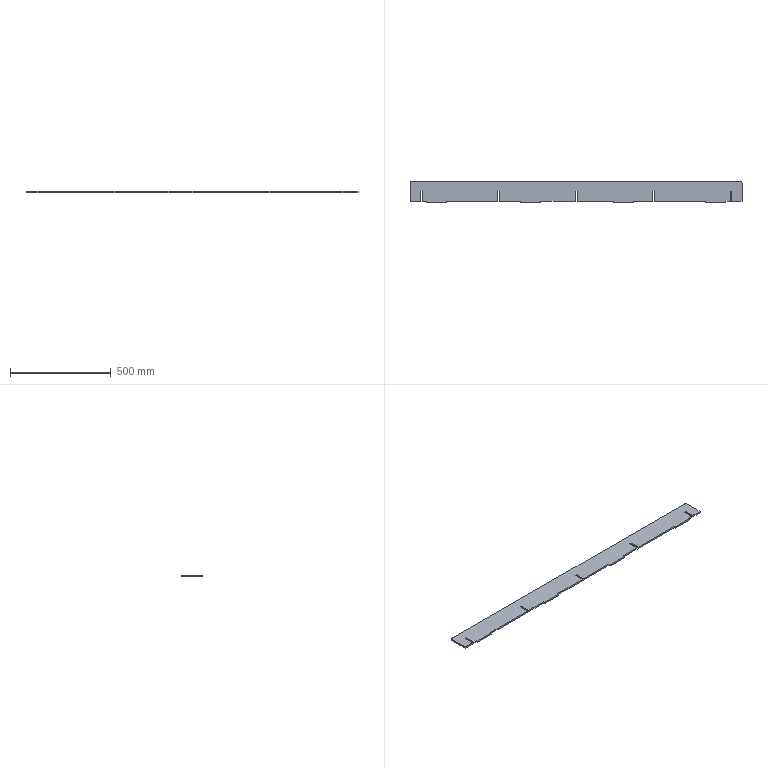Part | SolidWorks | features FlatPattern 1, SMBaseFlange 1, SheetMetal 1 | 1 solid | 44 faces | box 1650 x 107.5 x 8 mm | volume 1327497 mm3 | plane 42 | cylinder 2 | commonest cylinder face diameters 20 x2
STEP:
#1=CARTESIAN_POINT('',(838.136,-1279.45,0.));
#2=VERTEX_POINT('',#1);
#3=CARTESIAN_POINT('',(888.136,-1279.45,0.));
#4=VERTEX_POINT('',#3);
#5=CARTESIAN_POINT('',(838.136,-1279.45,0.));
#6=DIRECTION('',(1.,0.,0.));
#7=VECTOR('',#6,1000.);
#8=LINE('',#5,#7);
#9=EDGE_CURVE('',#2,#4,#8,.T.);
#10=ORIENTED_EDGE('',*,*,#9,.F.);
#11=CARTESIAN_POINT('',(838.136,-1279.45,-8.));
#12=VERTEX_POINT('',#11);
#13=CARTESIAN_POINT('',(838.136,-1279.45,-8.));
#14=DIRECTION('',(0.,0.,1.));
#15=VECTOR('',#14,1000.);
#16=LINE('',#13,#15);
#17=EDGE_CURVE('',#12,#2,#16,.T.);
#18=ORIENTED_EDGE('',*,*,#17,.F.);
#19=CARTESIAN_POINT('',(888.136,-1279.45,-8.));
#20=VERTEX_POINT('',#19);
#21=CARTESIAN_POINT('',(838.136,-1279.45,-8.));
#22=DIRECTION('',(1.,0.,0.));
#23=VECTOR('',#22,1000.);
#24=LINE('',#21,#23);
#25=EDGE_CURVE('',#12,#20,#24,.T.);
#26=ORIENTED_EDGE('',*,*,#25,.T.);
#27=CARTESIAN_POINT('',(888.136,-1279.45,-8.));
#28=DIRECTION('',(0.,0.,1.));
#29=VECTOR('',#28,1000.);
#30=LINE('',#27,#29);
#31=EDGE_CURVE('',#20,#4,#30,.T.);
#32=ORIENTED_EDGE('',*,*,#31,.T.);
#33=EDGE_LOOP('',(#10,#18,#26,#32));
#34=FACE_OUTER_BOUND('',#33,.T.);
#35=CARTESIAN_POINT('',(838.136,-1279.45,-8.));
#36=DIRECTION('',(0.,-1.,0.));
#37=DIRECTION('',(1.,0.,0.));
#38=AXIS2_PLACEMENT_3D('',#35,#36,#37);
#39=PLANE('',#38);
#40=ADVANCED_FACE('',(#34),#39,.T.);
#41=CARTESIAN_POINT('',(838.136,-1228.95,0.));
#42=VERTEX_POINT('',#41);
#43=CARTESIAN_POINT('',(838.136,-1279.45,0.));
#44=DIRECTION('',(0.,-1.,0.));
#45=VECTOR('',#44,1000.);
#46=LINE('',#43,#45);
#47=EDGE_CURVE('',#42,#2,#46,.T.);
#48=ORIENTED_EDGE('',*,*,#47,.F.);
#49=CARTESIAN_POINT('',(838.136,-1228.95,-8.));
#50=VERTEX_POINT('',#49);
#51=CARTESIAN_POINT('',(838.136,-1228.95,-8.));
#52=DIRECTION('',(0.,0.,1.));
#53=VECTOR('',#52,1000.);
#54=LINE('',#51,#53);
#55=EDGE_CURVE('',#50,#42,#54,.T.);
#56=ORIENTED_EDGE('',*,*,#55,.F.);
#57=CARTESIAN_POINT('',(838.136,-1279.45,-8.));
#58=DIRECTION('',(0.,-1.,0.));
#59=VECTOR('',#58,1000.);
#60=LINE('',#57,#59);
#61=EDGE_CURVE('',#50,#12,#60,.T.);
#62=ORIENTED_EDGE('',*,*,#61,.T.);
#63=ORIENTED_EDGE('',*,*,#17,.T.);
#64=EDGE_LOOP('',(#48,#56,#62,#63));
#65=FACE_OUTER_BOUND('',#64,.T.);
#66=CARTESIAN_POINT('',(838.136,-1279.45,-8.));
#67=DIRECTION('',(-1.,0.,0.));
#68=DIRECTION('',(0.,-1.,0.));
#69=AXIS2_PLACEMENT_3D('',#66,#67,#68);
#70=PLANE('',#69);
#71=ADVANCED_FACE('',(#65),#70,.T.);
#72=CARTESIAN_POINT('',(830.136,-1228.95,0.));
#73=VERTEX_POINT('',#72);
#74=CARTESIAN_POINT('',(838.136,-1228.95,0.));
#75=DIRECTION('',(1.,0.,0.));
#76=VECTOR('',#75,1000.);
#77=LINE('',#74,#76);
#78=EDGE_CURVE('',#73,#42,#77,.T.);
#79=ORIENTED_EDGE('',*,*,#78,.F.);
#80=CARTESIAN_POINT('',(830.136,-1228.95,-8.));
#81=VERTEX_POINT('',#80);
#82=CARTESIAN_POINT('',(830.136,-1228.95,-8.));
#83=DIRECTION('',(0.,0.,1.));
#84=VECTOR('',#83,1000.);
#85=LINE('',#82,#84);
#86=EDGE_CURVE('',#81,#73,#85,.T.);
#87=ORIENTED_EDGE('',*,*,#86,.F.);
#88=CARTESIAN_POINT('',(838.136,-1228.95,-8.));
#89=DIRECTION('',(1.,0.,0.));
#90=VECTOR('',#89,1000.);
#91=LINE('',#88,#90);
#92=EDGE_CURVE('',#81,#50,#91,.T.);
#93=ORIENTED_EDGE('',*,*,#92,.T.);
#94=ORIENTED_EDGE('',*,*,#55,.T.);
#95=EDGE_LOOP('',(#79,#87,#93,#94));
#96=FACE_OUTER_BOUND('',#95,.T.);
#97=CARTESIAN_POINT('',(838.136,-1228.95,-8.));
#98=DIRECTION('',(0.,-1.,0.));
#99=DIRECTION('',(0.,0.,-1.));
#100=AXIS2_PLACEMENT_3D('',#97,#98,#99);
#101=PLANE('',#100);
#102=ADVANCED_FACE('',(#96),#101,.T.);
#103=CARTESIAN_POINT('',(830.136,-1279.45,0.));
#104=VERTEX_POINT('',#103);
#105=CARTESIAN_POINT('',(830.136,-1228.95,0.));
#106=DIRECTION('',(0.,1.,0.));
#107=VECTOR('',#106,1000.);
#108=LINE('',#105,#107);
#109=EDGE_CURVE('',#104,#73,#108,.T.);
#110=ORIENTED_EDGE('',*,*,#109,.F.);
#111=CARTESIAN_POINT('',(830.136,-1279.45,-8.));
#112=VERTEX_POINT('',#111);
#113=CARTESIAN_POINT('',(830.136,-1279.45,-8.));
#114=DIRECTION('',(0.,0.,1.));
#115=VECTOR('',#114,1000.);
#116=LINE('',#113,#115);
#117=EDGE_CURVE('',#112,#104,#116,.T.);
#118=ORIENTED_EDGE('',*,*,#117,.F.);
#119=CARTESIAN_POINT('',(830.136,-1228.95,-8.));
#120=DIRECTION('',(0.,1.,0.));
#121=VECTOR('',#120,1000.);
#122=LINE('',#119,#121);
#123=EDGE_CURVE('',#112,#81,#122,.T.);
#124=ORIENTED_EDGE('',*,*,#123,.T.);
#125=ORIENTED_EDGE('',*,*,#86,.T.);
#126=EDGE_LOOP('',(#110,#118,#124,#125));
#127=FACE_OUTER_BOUND('',#126,.T.);
#128=CARTESIAN_POINT('',(830.136,-1228.95,-8.));
#129=DIRECTION('',(1.,0.,0.));
#130=DIRECTION('',(0.,0.,-1.));
#131=AXIS2_PLACEMENT_3D('',#128,#129,#130);
#132=PLANE('',#131);
#133=ADVANCED_FACE('',(#127),#132,.T.);
#134=CARTESIAN_POINT('',(808.136,-1279.45,0.));
#135=VERTEX_POINT('',#134);
#136=CARTESIAN_POINT('',(808.136,-1279.45,0.));
#137=DIRECTION('',(1.,0.,0.));
#138=VECTOR('',#137,1000.);
#139=LINE('',#136,#138);
#140=EDGE_CURVE('',#135,#104,#139,.T.);
#141=ORIENTED_EDGE('',*,*,#140,.F.);
#142=CARTESIAN_POINT('',(808.136,-1279.45,-8.));
#143=VERTEX_POINT('',#142);
#144=CARTESIAN_POINT('',(808.136,-1279.45,-8.));
#145=DIRECTION('',(0.,0.,1.));
#146=VECTOR('',#145,1000.);
#147=LINE('',#144,#146);
#148=EDGE_CURVE('',#143,#135,#147,.T.);
#149=ORIENTED_EDGE('',*,*,#148,.F.);
#150=CARTESIAN_POINT('',(808.136,-1279.45,-8.));
#151=DIRECTION('',(1.,0.,0.));
#152=VECTOR('',#151,1000.);
#153=LINE('',#150,#152);
#154=EDGE_CURVE('',#143,#112,#153,.T.);
#155=ORIENTED_EDGE('',*,*,#154,.T.);
#156=ORIENTED_EDGE('',*,*,#117,.T.);
#157=EDGE_LOOP('',(#141,#149,#155,#156));
#158=FACE_OUTER_BOUND('',#157,.T.);
#159=CARTESIAN_POINT('',(808.136,-1279.45,-8.));
#160=DIRECTION('',(0.,-1.,0.));
#161=DIRECTION('',(1.,0.,0.));
#162=AXIS2_PLACEMENT_3D('',#159,#160,#161);
#163=PLANE('',#162);
#164=ADVANCED_FACE('',(#158),#163,.T.);
#165=CARTESIAN_POINT('',(808.136,-1286.95,0.));
#166=VERTEX_POINT('',#165);
#167=CARTESIAN_POINT('',(808.136,-1279.45,0.));
#168=DIRECTION('',(0.,1.,0.));
#169=VECTOR('',#168,1000.);
#170=LINE('',#167,#169);
#171=EDGE_CURVE('',#166,#135,#170,.T.);
#172=ORIENTED_EDGE('',*,*,#171,.F.);
#173=CARTESIAN_POINT('',(808.136,-1286.95,-8.));
#174=VERTEX_POINT('',#173);
#175=CARTESIAN_POINT('',(808.136,-1286.95,-8.));
#176=DIRECTION('',(0.,0.,1.));
#177=VECTOR('',#176,1000.);
#178=LINE('',#175,#177);
#179=EDGE_CURVE('',#174,#166,#178,.T.);
#180=ORIENTED_EDGE('',*,*,#179,.F.);
#181=CARTESIAN_POINT('',(808.136,-1279.45,-8.));
#182=DIRECTION('',(0.,1.,0.));
#183=VECTOR('',#182,1000.);
#184=LINE('',#181,#183);
#185=EDGE_CURVE('',#174,#143,#184,.T.);
#186=ORIENTED_EDGE('',*,*,#185,.T.);
#187=ORIENTED_EDGE('',*,*,#148,.T.);
#188=EDGE_LOOP('',(#172,#180,#186,#187));
#189=FACE_OUTER_BOUND('',#188,.T.);
#190=CARTESIAN_POINT('',(808.136,-1279.45,-8.));
#191=DIRECTION('',(1.,0.,0.));
#192=DIRECTION('',(0.,0.,-1.));
#193=AXIS2_PLACEMENT_3D('',#190,#191,#192);
#194=PLANE('',#193);
#195=ADVANCED_FACE('',(#189),#194,.T.);
#196=CARTESIAN_POINT('',(708.136,-1286.95,0.));
#197=VERTEX_POINT('',#196);
#198=CARTESIAN_POINT('',(808.136,-1286.95,0.));
#199=DIRECTION('',(1.,0.,0.));
#200=VECTOR('',#199,1000.);
#201=LINE('',#198,#200);
#202=EDGE_CURVE('',#197,#166,#201,.T.);
#203=ORIENTED_EDGE('',*,*,#202,.F.);
#204=CARTESIAN_POINT('',(708.136,-1286.95,-8.));
#205=VERTEX_POINT('',#204);
#206=CARTESIAN_POINT('',(708.136,-1286.95,-8.));
#207=DIRECTION('',(0.,0.,1.));
#208=VECTOR('',#207,1000.);
#209=LINE('',#206,#208);
#210=EDGE_CURVE('',#205,#197,#209,.T.);
#211=ORIENTED_EDGE('',*,*,#210,.F.);
#212=CARTESIAN_POINT('',(808.136,-1286.95,-8.));
#213=DIRECTION('',(1.,0.,0.));
#214=VECTOR('',#213,1000.);
#215=LINE('',#212,#214);
#216=EDGE_CURVE('',#205,#174,#215,.T.);
#217=ORIENTED_EDGE('',*,*,#216,.T.);
#218=ORIENTED_EDGE('',*,*,#179,.T.);
#219=EDGE_LOOP('',(#203,#211,#217,#218));
#220=FACE_OUTER_BOUND('',#219,.T.);
#221=CARTESIAN_POINT('',(808.136,-1286.95,-8.));
#222=DIRECTION('',(0.,-1.,0.));
#223=DIRECTION('',(1.,0.,0.));
#224=AXIS2_PLACEMENT_3D('',#221,#222,#223);
#225=PLANE('',#224);
#226=ADVANCED_FACE('',(#220),#225,.T.);
#227=CARTESIAN_POINT('',(708.136,-1279.45,0.));
#228=VERTEX_POINT('',#227);
#229=CARTESIAN_POINT('',(708.136,-1286.95,0.));
#230=DIRECTION('',(0.,-1.,0.));
#231=VECTOR('',#230,1000.);
#232=LINE('',#229,#231);
#233=EDGE_CURVE('',#228,#197,#232,.T.);
#234=ORIENTED_EDGE('',*,*,#233,.F.);
#235=CARTESIAN_POINT('',(708.136,-1279.45,-8.));
#236=VERTEX_POINT('',#235);
#237=CARTESIAN_POINT('',(708.136,-1279.45,-8.));
#238=DIRECTION('',(0.,0.,1.));
#239=VECTOR('',#238,1000.);
#240=LINE('',#237,#239);
#241=EDGE_CURVE('',#236,#228,#240,.T.);
#242=ORIENTED_EDGE('',*,*,#241,.F.);
#243=CARTESIAN_POINT('',(708.136,-1286.95,-8.));
#244=DIRECTION('',(0.,-1.,0.));
#245=VECTOR('',#244,1000.);
#246=LINE('',#243,#245);
#247=EDGE_CURVE('',#236,#205,#246,.T.);
#248=ORIENTED_EDGE('',*,*,#247,.T.);
#249=ORIENTED_EDGE('',*,*,#210,.T.);
#250=EDGE_LOOP('',(#234,#242,#248,#249));
#251=FACE_OUTER_BOUND('',#250,.T.);
#252=CARTESIAN_POINT('',(708.136,-1286.95,-8.));
#253=DIRECTION('',(-1.,0.,0.));
#254=DIRECTION('',(0.,0.,1.));
#255=AXIS2_PLACEMENT_3D('',#252,#253,#254);
#256=PLANE('',#255);
#257=ADVANCED_FACE('',(#251),#256,.T.);
#258=CARTESIAN_POINT('',(453.136,-1279.45,0.));
#259=VERTEX_POINT('',#258);
#260=CARTESIAN_POINT('',(453.136,-1279.45,0.));
#261=DIRECTION('',(1.,0.,0.));
#262=VECTOR('',#261,1000.);
#263=LINE('',#260,#262);
#264=EDGE_CURVE('',#259,#228,#263,.T.);
#265=ORIENTED_EDGE('',*,*,#264,.F.);
#266=CARTESIAN_POINT('',(453.136,-1279.45,-8.));
#267=VERTEX_POINT('',#266);
#268=CARTESIAN_POINT('',(453.136,-1279.45,-8.));
#269=DIRECTION('',(0.,0.,1.));
#270=VECTOR('',#269,1000.);
#271=LINE('',#268,#270);
#272=EDGE_CURVE('',#267,#259,#271,.T.);
#273=ORIENTED_EDGE('',*,*,#272,.F.);
#274=CARTESIAN_POINT('',(453.136,-1279.45,-8.));
#275=DIRECTION('',(1.,0.,0.));
#276=VECTOR('',#275,1000.);
#277=LINE('',#274,#276);
#278=EDGE_CURVE('',#267,#236,#277,.T.);
#279=ORIENTED_EDGE('',*,*,#278,.T.);
#280=ORIENTED_EDGE('',*,*,#241,.T.);
#281=EDGE_LOOP('',(#265,#273,#279,#280));
#282=FACE_OUTER_BOUND('',#281,.T.);
#283=CARTESIAN_POINT('',(453.136,-1279.45,-8.));
#284=DIRECTION('',(0.,-1.,0.));
#285=DIRECTION('',(1.,0.,0.));
#286=AXIS2_PLACEMENT_3D('',#283,#284,#285);
#287=PLANE('',#286);
#288=ADVANCED_FACE('',(#282),#287,.T.);
#289=CARTESIAN_POINT('',(453.136,-1228.95,0.));
#290=VERTEX_POINT('',#289);
#291=CARTESIAN_POINT('',(453.136,-1279.45,0.));
#292=DIRECTION('',(0.,-1.,0.));
#293=VECTOR('',#292,1000.);
#294=LINE('',#291,#293);
#295=EDGE_CURVE('',#290,#259,#294,.T.);
#296=ORIENTED_EDGE('',*,*,#295,.F.);
#297=CARTESIAN_POINT('',(453.136,-1228.95,-8.));
#298=VERTEX_POINT('',#297);
#299=CARTESIAN_POINT('',(453.136,-1228.95,-8.));
#300=DIRECTION('',(0.,0.,1.));
#301=VECTOR('',#300,1000.);
#302=LINE('',#299,#301);
#303=EDGE_CURVE('',#298,#290,#302,.T.);
#304=ORIENTED_EDGE('',*,*,#303,.F.);
#305=CARTESIAN_POINT('',(453.136,-1279.45,-8.));
#306=DIRECTION('',(0.,-1.,0.));
#307=VECTOR('',#306,1000.);
#308=LINE('',#305,#307);
#309=EDGE_CURVE('',#298,#267,#308,.T.);
#310=ORIENTED_EDGE('',*,*,#309,.T.);
#311=ORIENTED_EDGE('',*,*,#272,.T.);
#312=EDGE_LOOP('',(#296,#304,#310,#311));
#313=FACE_OUTER_BOUND('',#312,.T.);
#314=CARTESIAN_POINT('',(453.136,-1279.45,-8.));
#315=DIRECTION('',(-1.,0.,0.));
#316=DIRECTION('',(0.,0.,1.));
#317=AXIS2_PLACEMENT_3D('',#314,#315,#316);
#318=PLANE('',#317);
#319=ADVANCED_FACE('',(#313),#318,.T.);
#320=CARTESIAN_POINT('',(445.136,-1228.95,0.));
#321=VERTEX_POINT('',#320);
#322=CARTESIAN_POINT('',(453.136,-1228.95,0.));
#323=DIRECTION('',(1.,0.,0.));
#324=VECTOR('',#323,1000.);
#325=LINE('',#322,#324);
#326=EDGE_CURVE('',#321,#290,#325,.T.);
#327=ORIENTED_EDGE('',*,*,#326,.F.);
#328=CARTESIAN_POINT('',(445.136,-1228.95,-8.));
#329=VERTEX_POINT('',#328);
#330=CARTESIAN_POINT('',(445.136,-1228.95,-8.));
#331=DIRECTION('',(0.,0.,1.));
#332=VECTOR('',#331,1000.);
#333=LINE('',#330,#332);
#334=EDGE_CURVE('',#329,#321,#333,.T.);
#335=ORIENTED_EDGE('',*,*,#334,.F.);
#336=CARTESIAN_POINT('',(453.136,-1228.95,-8.));
#337=DIRECTION('',(1.,0.,0.));
#338=VECTOR('',#337,1000.);
#339=LINE('',#336,#338);
#340=EDGE_CURVE('',#329,#298,#339,.T.);
#341=ORIENTED_EDGE('',*,*,#340,.T.);
#342=ORIENTED_EDGE('',*,*,#303,.T.);
#343=EDGE_LOOP('',(#327,#335,#341,#342));
#344=FACE_OUTER_BOUND('',#343,.T.);
#345=CARTESIAN_POINT('',(453.136,-1228.95,-8.));
#346=DIRECTION('',(0.,-1.,0.));
#347=DIRECTION('',(0.,0.,-1.));
#348=AXIS2_PLACEMENT_3D('',#345,#346,#347);
#349=PLANE('',#348);
#350=ADVANCED_FACE('',(#344),#349,.T.);
#351=CARTESIAN_POINT('',(445.136,-1279.45,0.));
#352=VERTEX_POINT('',#351);
#353=CARTESIAN_POINT('',(445.136,-1228.95,0.));
#354=DIRECTION('',(0.,1.,0.));
#355=VECTOR('',#354,1000.);
#356=LINE('',#353,#355);
#357=EDGE_CURVE('',#352,#321,#356,.T.);
#358=ORIENTED_EDGE('',*,*,#357,.F.);
#359=CARTESIAN_POINT('',(445.136,-1279.45,-8.));
#360=VERTEX_POINT('',#359);
#361=CARTESIAN_POINT('',(445.136,-1279.45,-8.));
#362=DIRECTION('',(0.,0.,1.));
#363=VECTOR('',#362,1000.);
#364=LINE('',#361,#363);
#365=EDGE_CURVE('',#360,#352,#364,.T.);
#366=ORIENTED_EDGE('',*,*,#365,.F.);
#367=CARTESIAN_POINT('',(445.136,-1228.95,-8.));
#368=DIRECTION('',(0.,1.,0.));
#369=VECTOR('',#368,1000.);
#370=LINE('',#367,#369);
#371=EDGE_CURVE('',#360,#329,#370,.T.);
#372=ORIENTED_EDGE('',*,*,#371,.T.);
#373=ORIENTED_EDGE('',*,*,#334,.T.);
#374=EDGE_LOOP('',(#358,#366,#372,#373));
#375=FACE_OUTER_BOUND('',#374,.T.);
#376=CARTESIAN_POINT('',(445.136,-1228.95,-8.));
#377=DIRECTION('',(1.,0.,0.));
#378=DIRECTION('',(0.,0.,-1.));
#379=AXIS2_PLACEMENT_3D('',#376,#377,#378);
#380=PLANE('',#379);
#381=ADVANCED_FACE('',(#375),#380,.T.);
#382=CARTESIAN_POINT('',(348.136,-1279.45,0.));
#383=VERTEX_POINT('',#382);
#384=CARTESIAN_POINT('',(348.136,-1279.45,0.));
#385=DIRECTION('',(1.,0.,0.));
#386=VECTOR('',#385,1000.);
#387=LINE('',#384,#386);
#388=EDGE_CURVE('',#383,#352,#387,.T.);
#389=ORIENTED_EDGE('',*,*,#388,.F.);
#390=CARTESIAN_POINT('',(348.136,-1279.45,-8.));
#391=VERTEX_POINT('',#390);
#392=CARTESIAN_POINT('',(348.136,-1279.45,-8.));
#393=DIRECTION('',(0.,0.,1.));
#394=VECTOR('',#393,1000.);
#395=LINE('',#392,#394);
#396=EDGE_CURVE('',#391,#383,#395,.T.);
#397=ORIENTED_EDGE('',*,*,#396,.F.);
#398=CARTESIAN_POINT('',(348.136,-1279.45,-8.));
#399=DIRECTION('',(1.,0.,0.));
#400=VECTOR('',#399,1000.);
#401=LINE('',#398,#400);
#402=EDGE_CURVE('',#391,#360,#401,.T.);
#403=ORIENTED_EDGE('',*,*,#402,.T.);
#404=ORIENTED_EDGE('',*,*,#365,.T.);
#405=EDGE_LOOP('',(#389,#397,#403,#404));
#406=FACE_OUTER_BOUND('',#405,.T.);
#407=CARTESIAN_POINT('',(348.136,-1279.45,-8.));
#408=DIRECTION('',(0.,-1.,0.));
#409=DIRECTION('',(1.,0.,0.));
#410=AXIS2_PLACEMENT_3D('',#407,#408,#409);
#411=PLANE('',#410);
#412=ADVANCED_FACE('',(#406),#411,.T.);
#413=CARTESIAN_POINT('',(348.136,-1286.95,0.));
#414=VERTEX_POINT('',#413);
#415=CARTESIAN_POINT('',(348.136,-1279.45,0.));
#416=DIRECTION('',(0.,1.,0.));
#417=VECTOR('',#416,1000.);
#418=LINE('',#415,#417);
#419=EDGE_CURVE('',#414,#383,#418,.T.);
#420=ORIENTED_EDGE('',*,*,#419,.F.);
#421=CARTESIAN_POINT('',(348.136,-1286.95,-8.));
#422=VERTEX_POINT('',#421);
#423=CARTESIAN_POINT('',(348.136,-1286.95,-8.));
#424=DIRECTION('',(0.,0.,1.));
#425=VECTOR('',#424,1000.);
#426=LINE('',#423,#425);
#427=EDGE_CURVE('',#422,#414,#426,.T.);
#428=ORIENTED_EDGE('',*,*,#427,.F.);
#429=CARTESIAN_POINT('',(348.136,-1279.45,-8.));
#430=DIRECTION('',(0.,1.,0.));
#431=VECTOR('',#430,1000.);
#432=LINE('',#429,#431);
#433=EDGE_CURVE('',#422,#391,#432,.T.);
#434=ORIENTED_EDGE('',*,*,#433,.T.);
#435=ORIENTED_EDGE('',*,*,#396,.T.);
#436=EDGE_LOOP('',(#420,#428,#434,#435));
#437=FACE_OUTER_BOUND('',#436,.T.);
#438=CARTESIAN_POINT('',(348.136,-1279.45,-8.));
#439=DIRECTION('',(1.,0.,0.));
#440=DIRECTION('',(0.,0.,-1.));
#441=AXIS2_PLACEMENT_3D('',#438,#439,#440);
#442=PLANE('',#441);
#443=ADVANCED_FACE('',(#437),#442,.T.);
#444=CARTESIAN_POINT('',(248.136,-1286.95,0.));
#445=VERTEX_POINT('',#444);
#446=CARTESIAN_POINT('',(348.136,-1286.95,0.));
#447=DIRECTION('',(1.,0.,0.));
#448=VECTOR('',#447,1000.);
#449=LINE('',#446,#448);
#450=EDGE_CURVE('',#445,#414,#449,.T.);
#451=ORIENTED_EDGE('',*,*,#450,.F.);
#452=CARTESIAN_POINT('',(248.136,-1286.95,-8.));
#453=VERTEX_POINT('',#452);
#454=CARTESIAN_POINT('',(248.136,-1286.95,-8.));
#455=DIRECTION('',(0.,0.,1.));
#456=VECTOR('',#455,1000.);
#457=LINE('',#454,#456);
#458=EDGE_CURVE('',#453,#445,#457,.T.);
#459=ORIENTED_EDGE('',*,*,#458,.F.);
#460=CARTESIAN_POINT('',(348.136,-1286.95,-8.));
#461=DIRECTION('',(1.,0.,0.));
#462=VECTOR('',#461,1000.);
#463=LINE('',#460,#462);
#464=EDGE_CURVE('',#453,#422,#463,.T.);
#465=ORIENTED_EDGE('',*,*,#464,.T.);
#466=ORIENTED_EDGE('',*,*,#427,.T.);
#467=EDGE_LOOP('',(#451,#459,#465,#466));
#468=FACE_OUTER_BOUND('',#467,.T.);
#469=CARTESIAN_POINT('',(348.136,-1286.95,-8.));
#470=DIRECTION('',(0.,-1.,0.));
#471=DIRECTION('',(0.,0.,-1.));
#472=AXIS2_PLACEMENT_3D('',#469,#470,#471);
#473=PLANE('',#472);
#474=ADVANCED_FACE('',(#468),#473,.T.);
#475=CARTESIAN_POINT('',(248.136,-1279.45,0.));
#476=VERTEX_POINT('',#475);
#477=CARTESIAN_POINT('',(248.136,-1286.95,0.));
#478=DIRECTION('',(0.,-1.,0.));
#479=VECTOR('',#478,1000.);
#480=LINE('',#477,#479);
#481=EDGE_CURVE('',#476,#445,#480,.T.);
#482=ORIENTED_EDGE('',*,*,#481,.F.);
#483=CARTESIAN_POINT('',(248.136,-1279.45,-8.));
#484=VERTEX_POINT('',#483);
#485=CARTESIAN_POINT('',(248.136,-1279.45,-8.));
#486=DIRECTION('',(0.,0.,1.));
#487=VECTOR('',#486,1000.);
#488=LINE('',#485,#487);
#489=EDGE_CURVE('',#484,#476,#488,.T.);
#490=ORIENTED_EDGE('',*,*,#489,.F.);
#491=CARTESIAN_POINT('',(248.136,-1286.95,-8.));
#492=DIRECTION('',(0.,-1.,0.));
#493=VECTOR('',#492,1000.);
#494=LINE('',#491,#493);
#495=EDGE_CURVE('',#484,#453,#494,.T.);
#496=ORIENTED_EDGE('',*,*,#495,.T.);
#497=ORIENTED_EDGE('',*,*,#458,.T.);
#498=EDGE_LOOP('',(#482,#490,#496,#497));
#499=FACE_OUTER_BOUND('',#498,.T.);
#500=CARTESIAN_POINT('',(248.136,-1286.95,-8.));
#501=DIRECTION('',(-1.,0.,0.));
#502=DIRECTION('',(0.,0.,1.));
#503=AXIS2_PLACEMENT_3D('',#500,#501,#502);
#504=PLANE('',#503);
#505=ADVANCED_FACE('',(#499),#504,.T.);
#506=CARTESIAN_POINT('',(68.136,-1279.45,0.));
#507=VERTEX_POINT('',#506);
#508=CARTESIAN_POINT('',(68.136,-1279.45,0.));
#509=DIRECTION('',(1.,0.,0.));
#510=VECTOR('',#509,1000.);
#511=LINE('',#508,#510);
#512=EDGE_CURVE('',#507,#476,#511,.T.);
#513=ORIENTED_EDGE('',*,*,#512,.F.);
#514=CARTESIAN_POINT('',(68.136,-1279.45,-8.));
#515=VERTEX_POINT('',#514);
#516=CARTESIAN_POINT('',(68.136,-1279.45,-8.));
#517=DIRECTION('',(0.,0.,1.));
#518=VECTOR('',#517,1000.);
#519=LINE('',#516,#518);
#520=EDGE_CURVE('',#515,#507,#519,.T.);
#521=ORIENTED_EDGE('',*,*,#520,.F.);
#522=CARTESIAN_POINT('',(68.136,-1279.45,-8.));
#523=DIRECTION('',(1.,0.,0.));
#524=VECTOR('',#523,1000.);
#525=LINE('',#522,#524);
#526=EDGE_CURVE('',#515,#484,#525,.T.);
#527=ORIENTED_EDGE('',*,*,#526,.T.);
#528=ORIENTED_EDGE('',*,*,#489,.T.);
#529=EDGE_LOOP('',(#513,#521,#527,#528));
#530=FACE_OUTER_BOUND('',#529,.T.);
#531=CARTESIAN_POINT('',(68.136,-1279.45,-8.));
#532=DIRECTION('',(0.,-1.,0.));
#533=DIRECTION('',(1.,0.,0.));
#534=AXIS2_PLACEMENT_3D('',#531,#532,#533);
#535=PLANE('',#534);
#536=ADVANCED_FACE('',(#530),#535,.T.);
#537=CARTESIAN_POINT('',(68.136,-1228.95,0.));
#538=VERTEX_POINT('',#537);
#539=CARTESIAN_POINT('',(68.136,-1279.45,0.));
#540=DIRECTION('',(0.,-1.,0.));
#541=VECTOR('',#540,1000.);
#542=LINE('',#539,#541);
#543=EDGE_CURVE('',#538,#507,#542,.T.);
#544=ORIENTED_EDGE('',*,*,#543,.F.);
#545=CARTESIAN_POINT('',(68.136,-1228.95,-8.));
#546=VERTEX_POINT('',#545);
#547=CARTESIAN_POINT('',(68.136,-1228.95,-8.));
#548=DIRECTION('',(0.,0.,1.));
#549=VECTOR('',#548,1000.);
#550=LINE('',#547,#549);
#551=EDGE_CURVE('',#546,#538,#550,.T.);
#552=ORIENTED_EDGE('',*,*,#551,.F.);
#553=CARTESIAN_POINT('',(68.136,-1279.45,-8.));
#554=DIRECTION('',(0.,-1.,0.));
#555=VECTOR('',#554,1000.);
#556=LINE('',#553,#555);
#557=EDGE_CURVE('',#546,#515,#556,.T.);
#558=ORIENTED_EDGE('',*,*,#557,.T.);
#559=ORIENTED_EDGE('',*,*,#520,.T.);
#560=EDGE_LOOP('',(#544,#552,#558,#559));
#561=FACE_OUTER_BOUND('',#560,.T.);
#562=CARTESIAN_POINT('',(68.136,-1279.45,-8.));
#563=DIRECTION('',(-1.,0.,0.));
#564=DIRECTION('',(0.,0.,1.));
#565=AXIS2_PLACEMENT_3D('',#562,#563,#564);
#566=PLANE('',#565);
#567=ADVANCED_FACE('',(#561),#566,.T.);
#568=CARTESIAN_POINT('',(60.136,-1228.95,0.));
#569=VERTEX_POINT('',#568);
#570=CARTESIAN_POINT('',(68.136,-1228.95,0.));
#571=DIRECTION('',(1.,0.,0.));
#572=VECTOR('',#571,1000.);
#573=LINE('',#570,#572);
#574=EDGE_CURVE('',#569,#538,#573,.T.);
#575=ORIENTED_EDGE('',*,*,#574,.F.);
#576=CARTESIAN_POINT('',(60.136,-1228.95,-8.));
#577=VERTEX_POINT('',#576);
#578=CARTESIAN_POINT('',(60.136,-1228.95,-8.));
#579=DIRECTION('',(0.,0.,1.));
#580=VECTOR('',#579,1000.);
#581=LINE('',#578,#580);
#582=EDGE_CURVE('',#577,#569,#581,.T.);
#583=ORIENTED_EDGE('',*,*,#582,.F.);
#584=CARTESIAN_POINT('',(68.136,-1228.95,-8.));
#585=DIRECTION('',(1.,0.,0.));
#586=VECTOR('',#585,1000.);
#587=LINE('',#584,#586);
#588=EDGE_CURVE('',#577,#546,#587,.T.);
#589=ORIENTED_EDGE('',*,*,#588,.T.);
#590=ORIENTED_EDGE('',*,*,#551,.T.);
#591=EDGE_LOOP('',(#575,#583,#589,#590));
#592=FACE_OUTER_BOUND('',#591,.T.);
#593=CARTESIAN_POINT('',(68.136,-1228.95,-8.));
#594=DIRECTION('',(0.,-1.,0.));
#595=DIRECTION('',(0.,0.,-1.));
#596=AXIS2_PLACEMENT_3D('',#593,#594,#595);
#597=PLANE('',#596);
#598=ADVANCED_FACE('',(#592),#597,.T.);
#599=CARTESIAN_POINT('',(60.136,-1279.45,0.));
#600=VERTEX_POINT('',#599);
#601=CARTESIAN_POINT('',(60.136,-1228.95,0.));
#602=DIRECTION('',(0.,1.,0.));
#603=VECTOR('',#602,1000.);
#604=LINE('',#601,#603);
#605=EDGE_CURVE('',#600,#569,#604,.T.);
#606=ORIENTED_EDGE('',*,*,#605,.F.);
#607=CARTESIAN_POINT('',(60.136,-1279.45,-8.));
#608=VERTEX_POINT('',#607);
#609=CARTESIAN_POINT('',(60.136,-1279.45,-8.));
#610=DIRECTION('',(0.,0.,1.));
#611=VECTOR('',#610,1000.);
#612=LINE('',#609,#611);
#613=EDGE_CURVE('',#608,#600,#612,.T.);
#614=ORIENTED_EDGE('',*,*,#613,.F.);
#615=CARTESIAN_POINT('',(60.136,-1228.95,-8.));
#616=DIRECTION('',(0.,1.,0.));
#617=VECTOR('',#616,1000.);
#618=LINE('',#615,#617);
#619=EDGE_CURVE('',#608,#577,#618,.T.);
#620=ORIENTED_EDGE('',*,*,#619,.T.);
#621=ORIENTED_EDGE('',*,*,#582,.T.);
#622=EDGE_LOOP('',(#606,#614,#620,#621));
#623=FACE_OUTER_BOUND('',#622,.T.);
#624=CARTESIAN_POINT('',(60.136,-1228.95,-8.));
#625=DIRECTION('',(1.,0.,0.));
#626=DIRECTION('',(0.,0.,-1.));
#627=AXIS2_PLACEMENT_3D('',#624,#625,#626);
#628=PLANE('',#627);
#629=ADVANCED_FACE('',(#623),#628,.T.);
#630=CARTESIAN_POINT('',(-111.864,-1279.45,0.));
#631=VERTEX_POINT('',#630);
#632=CARTESIAN_POINT('',(-111.864,-1279.45,0.));
#633=DIRECTION('',(1.,0.,0.));
#634=VECTOR('',#633,1000.);
#635=LINE('',#632,#634);
#636=EDGE_CURVE('',#631,#600,#635,.T.);
#637=ORIENTED_EDGE('',*,*,#636,.F.);
#638=CARTESIAN_POINT('',(-111.864,-1279.45,-8.));
#639=VERTEX_POINT('',#638);
#640=CARTESIAN_POINT('',(-111.864,-1279.45,-8.));
#641=DIRECTION('',(0.,0.,1.));
#642=VECTOR('',#641,1000.);
#643=LINE('',#640,#642);
#644=EDGE_CURVE('',#639,#631,#643,.T.);
#645=ORIENTED_EDGE('',*,*,#644,.F.);
#646=CARTESIAN_POINT('',(-111.864,-1279.45,-8.));
#647=DIRECTION('',(1.,0.,0.));
#648=VECTOR('',#647,1000.);
#649=LINE('',#646,#648);
#650=EDGE_CURVE('',#639,#608,#649,.T.);
#651=ORIENTED_EDGE('',*,*,#650,.T.);
#652=ORIENTED_EDGE('',*,*,#613,.T.);
#653=EDGE_LOOP('',(#637,#645,#651,#652));
#654=FACE_OUTER_BOUND('',#653,.T.);
#655=CARTESIAN_POINT('',(-111.864,-1279.45,-8.));
#656=DIRECTION('',(0.,-1.,0.));
#657=DIRECTION('',(1.,0.,0.));
#658=AXIS2_PLACEMENT_3D('',#655,#656,#657);
#659=PLANE('',#658);
#660=ADVANCED_FACE('',(#654),#659,.T.);
#661=CARTESIAN_POINT('',(-111.864,-1286.95,0.));
#662=VERTEX_POINT('',#661);
#663=CARTESIAN_POINT('',(-111.864,-1279.45,0.));
#664=DIRECTION('',(0.,1.,0.));
#665=VECTOR('',#664,1000.);
#666=LINE('',#663,#665);
#667=EDGE_CURVE('',#662,#631,#666,.T.);
#668=ORIENTED_EDGE('',*,*,#667,.F.);
#669=CARTESIAN_POINT('',(-111.864,-1286.95,-8.));
#670=VERTEX_POINT('',#669);
#671=CARTESIAN_POINT('',(-111.864,-1286.95,-8.));
#672=DIRECTION('',(0.,0.,1.));
#673=VECTOR('',#672,1000.);
#674=LINE('',#671,#673);
#675=EDGE_CURVE('',#670,#662,#674,.T.);
#676=ORIENTED_EDGE('',*,*,#675,.F.);
#677=CARTESIAN_POINT('',(-111.864,-1279.45,-8.));
#678=DIRECTION('',(0.,1.,0.));
#679=VECTOR('',#678,1000.);
#680=LINE('',#677,#679);
#681=EDGE_CURVE('',#670,#639,#680,.T.);
#682=ORIENTED_EDGE('',*,*,#681,.T.);
#683=ORIENTED_EDGE('',*,*,#644,.T.);
#684=EDGE_LOOP('',(#668,#676,#682,#683));
#685=FACE_OUTER_BOUND('',#684,.T.);
#686=CARTESIAN_POINT('',(-111.864,-1279.45,-8.));
#687=DIRECTION('',(1.,0.,0.));
#688=DIRECTION('',(0.,0.,-1.));
#689=AXIS2_PLACEMENT_3D('',#686,#687,#688);
#690=PLANE('',#689);
#691=ADVANCED_FACE('',(#685),#690,.T.);
#692=CARTESIAN_POINT('',(-211.864,-1286.95,0.));
#693=VERTEX_POINT('',#692);
#694=CARTESIAN_POINT('',(-111.864,-1286.95,0.));
#695=DIRECTION('',(1.,0.,0.));
#696=VECTOR('',#695,1000.);
#697=LINE('',#694,#696);
#698=EDGE_CURVE('',#693,#662,#697,.T.);
#699=ORIENTED_EDGE('',*,*,#698,.F.);
#700=CARTESIAN_POINT('',(-211.864,-1286.95,-8.));
#701=VERTEX_POINT('',#700);
#702=CARTESIAN_POINT('',(-211.864,-1286.95,-8.));
#703=DIRECTION('',(0.,0.,1.));
#704=VECTOR('',#703,1000.);
#705=LINE('',#702,#704);
#706=EDGE_CURVE('',#701,#693,#705,.T.);
#707=ORIENTED_EDGE('',*,*,#706,.F.);
#708=CARTESIAN_POINT('',(-111.864,-1286.95,-8.));
#709=DIRECTION('',(1.,0.,0.));
#710=VECTOR('',#709,1000.);
#711=LINE('',#708,#710);
#712=EDGE_CURVE('',#701,#670,#711,.T.);
#713=ORIENTED_EDGE('',*,*,#712,.T.);
#714=ORIENTED_EDGE('',*,*,#675,.T.);
#715=EDGE_LOOP('',(#699,#707,#713,#714));
#716=FACE_OUTER_BOUND('',#715,.T.);
#717=CARTESIAN_POINT('',(-111.864,-1286.95,-8.));
#718=DIRECTION('',(0.,-1.,0.));
#719=DIRECTION('',(0.,0.,-1.));
#720=AXIS2_PLACEMENT_3D('',#717,#718,#719);
#721=PLANE('',#720);
#722=ADVANCED_FACE('',(#716),#721,.T.);
#723=CARTESIAN_POINT('',(-211.864,-1279.45,0.));
#724=VERTEX_POINT('',#723);
#725=CARTESIAN_POINT('',(-211.864,-1286.95,0.));
#726=DIRECTION('',(0.,-1.,0.));
#727=VECTOR('',#726,1000.);
#728=LINE('',#725,#727);
#729=EDGE_CURVE('',#724,#693,#728,.T.);
#730=ORIENTED_EDGE('',*,*,#729,.F.);
#731=CARTESIAN_POINT('',(-211.864,-1279.45,-8.));
#732=VERTEX_POINT('',#731);
#733=CARTESIAN_POINT('',(-211.864,-1279.45,-8.));
#734=DIRECTION('',(0.,0.,1.));
#735=VECTOR('',#734,1000.);
#736=LINE('',#733,#735);
#737=EDGE_CURVE('',#732,#724,#736,.T.);
#738=ORIENTED_EDGE('',*,*,#737,.F.);
#739=CARTESIAN_POINT('',(-211.864,-1286.95,-8.));
#740=DIRECTION('',(0.,-1.,0.));
#741=VECTOR('',#740,1000.);
#742=LINE('',#739,#741);
#743=EDGE_CURVE('',#732,#701,#742,.T.);
#744=ORIENTED_EDGE('',*,*,#743,.T.);
#745=ORIENTED_EDGE('',*,*,#706,.T.);
#746=EDGE_LOOP('',(#730,#738,#744,#745));
#747=FACE_OUTER_BOUND('',#746,.T.);
#748=CARTESIAN_POINT('',(-211.864,-1286.95,-8.));
#749=DIRECTION('',(-1.,0.,0.));
#750=DIRECTION('',(0.,0.,1.));
#751=AXIS2_PLACEMENT_3D('',#748,#749,#750);
#752=PLANE('',#751);
#753=ADVANCED_FACE('',(#747),#752,.T.);
#754=CARTESIAN_POINT('',(-316.864,-1279.45,0.));
#755=VERTEX_POINT('',#754);
#756=CARTESIAN_POINT('',(-316.864,-1279.45,0.));
#757=DIRECTION('',(1.,0.,0.));
#758=VECTOR('',#757,1000.);
#759=LINE('',#756,#758);
#760=EDGE_CURVE('',#755,#724,#759,.T.);
#761=ORIENTED_EDGE('',*,*,#760,.F.);
#762=CARTESIAN_POINT('',(-316.864,-1279.45,-8.));
#763=VERTEX_POINT('',#762);
#764=CARTESIAN_POINT('',(-316.864,-1279.45,-8.));
#765=DIRECTION('',(0.,0.,1.));
#766=VECTOR('',#765,1000.);
#767=LINE('',#764,#766);
#768=EDGE_CURVE('',#763,#755,#767,.T.);
#769=ORIENTED_EDGE('',*,*,#768,.F.);
#770=CARTESIAN_POINT('',(-316.864,-1279.45,-8.));
#771=DIRECTION('',(1.,0.,0.));
#772=VECTOR('',#771,1000.);
#773=LINE('',#770,#772);
#774=EDGE_CURVE('',#763,#732,#773,.T.);
#775=ORIENTED_EDGE('',*,*,#774,.T.);
#776=ORIENTED_EDGE('',*,*,#737,.T.);
#777=EDGE_LOOP('',(#761,#769,#775,#776));
#778=FACE_OUTER_BOUND('',#777,.T.);
#779=CARTESIAN_POINT('',(-316.864,-1279.45,-8.));
#780=DIRECTION('',(0.,-1.,0.));
#781=DIRECTION('',(1.,0.,0.));
#782=AXIS2_PLACEMENT_3D('',#779,#780,#781);
#783=PLANE('',#782);
#784=ADVANCED_FACE('',(#778),#783,.T.);
#785=CARTESIAN_POINT('',(-316.864,-1228.95,0.));
#786=VERTEX_POINT('',#785);
#787=CARTESIAN_POINT('',(-316.864,-1279.45,0.));
#788=DIRECTION('',(0.,-1.,0.));
#789=VECTOR('',#788,1000.);
#790=LINE('',#787,#789);
#791=EDGE_CURVE('',#786,#755,#790,.T.);
#792=ORIENTED_EDGE('',*,*,#791,.F.);
#793=CARTESIAN_POINT('',(-316.864,-1228.95,-8.));
#794=VERTEX_POINT('',#793);
#795=CARTESIAN_POINT('',(-316.864,-1228.95,-8.));
#796=DIRECTION('',(0.,0.,1.));
#797=VECTOR('',#796,1000.);
#798=LINE('',#795,#797);
#799=EDGE_CURVE('',#794,#786,#798,.T.);
#800=ORIENTED_EDGE('',*,*,#799,.F.);
#801=CARTESIAN_POINT('',(-316.864,-1279.45,-8.));
#802=DIRECTION('',(0.,-1.,0.));
#803=VECTOR('',#802,1000.);
#804=LINE('',#801,#803);
#805=EDGE_CURVE('',#794,#763,#804,.T.);
#806=ORIENTED_EDGE('',*,*,#805,.T.);
#807=ORIENTED_EDGE('',*,*,#768,.T.);
#808=EDGE_LOOP('',(#792,#800,#806,#807));
#809=FACE_OUTER_BOUND('',#808,.T.);
#810=CARTESIAN_POINT('',(-316.864,-1279.45,-8.));
#811=DIRECTION('',(-1.,0.,0.));
#812=DIRECTION('',(0.,0.,1.));
#813=AXIS2_PLACEMENT_3D('',#810,#811,#812);
#814=PLANE('',#813);
#815=ADVANCED_FACE('',(#809),#814,.T.);
#816=CARTESIAN_POINT('',(-324.864,-1228.95,0.));
#817=VERTEX_POINT('',#816);
#818=CARTESIAN_POINT('',(-316.864,-1228.95,0.));
#819=DIRECTION('',(1.,0.,0.));
#820=VECTOR('',#819,1000.);
#821=LINE('',#818,#820);
#822=EDGE_CURVE('',#817,#786,#821,.T.);
#823=ORIENTED_EDGE('',*,*,#822,.F.);
#824=CARTESIAN_POINT('',(-324.864,-1228.95,-8.));
#825=VERTEX_POINT('',#824);
#826=CARTESIAN_POINT('',(-324.864,-1228.95,-8.));
#827=DIRECTION('',(0.,0.,1.));
#828=VECTOR('',#827,1000.);
#829=LINE('',#826,#828);
#830=EDGE_CURVE('',#825,#817,#829,.T.);
#831=ORIENTED_EDGE('',*,*,#830,.F.);
#832=CARTESIAN_POINT('',(-316.864,-1228.95,-8.));
#833=DIRECTION('',(1.,0.,0.));
#834=VECTOR('',#833,1000.);
#835=LINE('',#832,#834);
#836=EDGE_CURVE('',#825,#794,#835,.T.);
#837=ORIENTED_EDGE('',*,*,#836,.T.);
#838=ORIENTED_EDGE('',*,*,#799,.T.);
#839=EDGE_LOOP('',(#823,#831,#837,#838));
#840=FACE_OUTER_BOUND('',#839,.T.);
#841=CARTESIAN_POINT('',(-316.864,-1228.95,-8.));
#842=DIRECTION('',(0.,-1.,0.));
#843=DIRECTION('',(0.,0.,-1.));
#844=AXIS2_PLACEMENT_3D('',#841,#842,#843);
#845=PLANE('',#844);
#846=ADVANCED_FACE('',(#840),#845,.T.);
#847=CARTESIAN_POINT('',(-324.864,-1279.45,0.));
#848=VERTEX_POINT('',#847);
#849=CARTESIAN_POINT('',(-324.864,-1228.95,0.));
#850=DIRECTION('',(0.,1.,0.));
#851=VECTOR('',#850,1000.);
#852=LINE('',#849,#851);
#853=EDGE_CURVE('',#848,#817,#852,.T.);
#854=ORIENTED_EDGE('',*,*,#853,.F.);
#855=CARTESIAN_POINT('',(-324.864,-1279.45,-8.));
#856=VERTEX_POINT('',#855);
#857=CARTESIAN_POINT('',(-324.864,-1279.45,-8.));
#858=DIRECTION('',(0.,0.,1.));
#859=VECTOR('',#858,1000.);
#860=LINE('',#857,#859);
#861=EDGE_CURVE('',#856,#848,#860,.T.);
#862=ORIENTED_EDGE('',*,*,#861,.F.);
#863=CARTESIAN_POINT('',(-324.864,-1228.95,-8.));
#864=DIRECTION('',(0.,1.,0.));
#865=VECTOR('',#864,1000.);
#866=LINE('',#863,#865);
#867=EDGE_CURVE('',#856,#825,#866,.T.);
#868=ORIENTED_EDGE('',*,*,#867,.T.);
#869=ORIENTED_EDGE('',*,*,#830,.T.);
#870=EDGE_LOOP('',(#854,#862,#868,#869));
#871=FACE_OUTER_BOUND('',#870,.T.);
#872=CARTESIAN_POINT('',(-324.864,-1228.95,-8.));
#873=DIRECTION('',(1.,0.,0.));
#874=DIRECTION('',(0.,0.,-1.));
#875=AXIS2_PLACEMENT_3D('',#872,#873,#874);
#876=PLANE('',#875);
#877=ADVANCED_FACE('',(#871),#876,.T.);
#878=CARTESIAN_POINT('',(-581.864,-1279.45,0.));
#879=VERTEX_POINT('',#878);
#880=CARTESIAN_POINT('',(-581.864,-1279.45,0.));
#881=DIRECTION('',(1.,0.,0.));
#882=VECTOR('',#881,1000.);
#883=LINE('',#880,#882);
#884=EDGE_CURVE('',#879,#848,#883,.T.);
#885=ORIENTED_EDGE('',*,*,#884,.F.);
#886=CARTESIAN_POINT('',(-581.864,-1279.45,-8.));
#887=VERTEX_POINT('',#886);
#888=CARTESIAN_POINT('',(-581.864,-1279.45,-8.));
#889=DIRECTION('',(0.,0.,1.));
#890=VECTOR('',#889,1000.);
#891=LINE('',#888,#890);
#892=EDGE_CURVE('',#887,#879,#891,.T.);
#893=ORIENTED_EDGE('',*,*,#892,.F.);
#894=CARTESIAN_POINT('',(-581.864,-1279.45,-8.));
#895=DIRECTION('',(1.,0.,0.));
#896=VECTOR('',#895,1000.);
#897=LINE('',#894,#896);
#898=EDGE_CURVE('',#887,#856,#897,.T.);
#899=ORIENTED_EDGE('',*,*,#898,.T.);
#900=ORIENTED_EDGE('',*,*,#861,.T.);
#901=EDGE_LOOP('',(#885,#893,#899,#900));
#902=FACE_OUTER_BOUND('',#901,.T.);
#903=CARTESIAN_POINT('',(-581.864,-1279.45,-8.));
#904=DIRECTION('',(0.,-1.,0.));
#905=DIRECTION('',(1.,0.,0.));
#906=AXIS2_PLACEMENT_3D('',#903,#904,#905);
#907=PLANE('',#906);
#908=ADVANCED_FACE('',(#902),#907,.T.);
#909=CARTESIAN_POINT('',(-581.864,-1286.95,0.));
#910=VERTEX_POINT('',#909);
#911=CARTESIAN_POINT('',(-581.864,-1279.45,0.));
#912=DIRECTION('',(0.,1.,0.));
#913=VECTOR('',#912,1000.);
#914=LINE('',#911,#913);
#915=EDGE_CURVE('',#910,#879,#914,.T.);
#916=ORIENTED_EDGE('',*,*,#915,.F.);
#917=CARTESIAN_POINT('',(-581.864,-1286.95,-8.));
#918=VERTEX_POINT('',#917);
#919=CARTESIAN_POINT('',(-581.864,-1286.95,-8.));
#920=DIRECTION('',(0.,0.,1.));
#921=VECTOR('',#920,1000.);
#922=LINE('',#919,#921);
#923=EDGE_CURVE('',#918,#910,#922,.T.);
#924=ORIENTED_EDGE('',*,*,#923,.F.);
#925=CARTESIAN_POINT('',(-581.864,-1279.45,-8.));
#926=DIRECTION('',(0.,1.,0.));
#927=VECTOR('',#926,1000.);
#928=LINE('',#925,#927);
#929=EDGE_CURVE('',#918,#887,#928,.T.);
#930=ORIENTED_EDGE('',*,*,#929,.T.);
#931=ORIENTED_EDGE('',*,*,#892,.T.);
#932=EDGE_LOOP('',(#916,#924,#930,#931));
#933=FACE_OUTER_BOUND('',#932,.T.);
#934=CARTESIAN_POINT('',(-581.864,-1279.45,-8.));
#935=DIRECTION('',(1.,0.,0.));
#936=DIRECTION('',(0.,0.,-1.));
#937=AXIS2_PLACEMENT_3D('',#934,#935,#936);
#938=PLANE('',#937);
#939=ADVANCED_FACE('',(#933),#938,.T.);
#940=CARTESIAN_POINT('',(-681.864,-1286.95,0.));
#941=VERTEX_POINT('',#940);
#942=CARTESIAN_POINT('',(-581.864,-1286.95,0.));
#943=DIRECTION('',(1.,0.,0.));
#944=VECTOR('',#943,1000.);
#945=LINE('',#942,#944);
#946=EDGE_CURVE('',#941,#910,#945,.T.);
#947=ORIENTED_EDGE('',*,*,#946,.F.);
#948=CARTESIAN_POINT('',(-681.864,-1286.95,-8.));
#949=VERTEX_POINT('',#948);
#950=CARTESIAN_POINT('',(-681.864,-1286.95,-8.));
#951=DIRECTION('',(0.,0.,1.));
#952=VECTOR('',#951,1000.);
#953=LINE('',#950,#952);
#954=EDGE_CURVE('',#949,#941,#953,.T.);
#955=ORIENTED_EDGE('',*,*,#954,.F.);
#956=CARTESIAN_POINT('',(-581.864,-1286.95,-8.));
#957=DIRECTION('',(1.,0.,0.));
#958=VECTOR('',#957,1000.);
#959=LINE('',#956,#958);
#960=EDGE_CURVE('',#949,#918,#959,.T.);
#961=ORIENTED_EDGE('',*,*,#960,.T.);
#962=ORIENTED_EDGE('',*,*,#923,.T.);
#963=EDGE_LOOP('',(#947,#955,#961,#962));
#964=FACE_OUTER_BOUND('',#963,.T.);
#965=CARTESIAN_POINT('',(-581.864,-1286.95,-8.));
#966=DIRECTION('',(0.,-1.,0.));
#967=DIRECTION('',(1.,0.,0.));
#968=AXIS2_PLACEMENT_3D('',#965,#966,#967);
#969=PLANE('',#968);
#970=ADVANCED_FACE('',(#964),#969,.T.);
#971=CARTESIAN_POINT('',(-681.864,-1279.45,0.));
#972=VERTEX_POINT('',#971);
#973=CARTESIAN_POINT('',(-681.864,-1286.95,0.));
#974=DIRECTION('',(0.,-1.,0.));
#975=VECTOR('',#974,1000.);
#976=LINE('',#973,#975);
#977=EDGE_CURVE('',#972,#941,#976,.T.);
#978=ORIENTED_EDGE('',*,*,#977,.F.);
#979=CARTESIAN_POINT('',(-681.864,-1279.45,-8.));
#980=VERTEX_POINT('',#979);
#981=CARTESIAN_POINT('',(-681.864,-1279.45,-8.));
#982=DIRECTION('',(0.,0.,1.));
#983=VECTOR('',#982,1000.);
#984=LINE('',#981,#983);
#985=EDGE_CURVE('',#980,#972,#984,.T.);
#986=ORIENTED_EDGE('',*,*,#985,.F.);
#987=CARTESIAN_POINT('',(-681.864,-1286.95,-8.));
#988=DIRECTION('',(0.,-1.,0.));
#989=VECTOR('',#988,1000.);
#990=LINE('',#987,#989);
#991=EDGE_CURVE('',#980,#949,#990,.T.);
#992=ORIENTED_EDGE('',*,*,#991,.T.);
#993=ORIENTED_EDGE('',*,*,#954,.T.);
#994=EDGE_LOOP('',(#978,#986,#992,#993));
#995=FACE_OUTER_BOUND('',#994,.T.);
#996=CARTESIAN_POINT('',(-681.864,-1286.95,-8.));
#997=DIRECTION('',(-1.,0.,0.));
#998=DIRECTION('',(0.,0.,1.));
#999=AXIS2_PLACEMENT_3D('',#996,#997,#998);
#1000=PLANE('',#999);
#1001=ADVANCED_FACE('',(#995),#1000,.T.);
#1002=CARTESIAN_POINT('',(-701.864,-1279.45,0.));
#1003=VERTEX_POINT('',#1002);
#1004=CARTESIAN_POINT('',(-701.864,-1279.45,0.));
#1005=DIRECTION('',(1.,0.,0.));
#1006=VECTOR('',#1005,1000.);
#1007=LINE('',#1004,#1006);
#1008=EDGE_CURVE('',#1003,#972,#1007,.T.);
#1009=ORIENTED_EDGE('',*,*,#1008,.F.);
#1010=CARTESIAN_POINT('',(-701.864,-1279.45,-8.));
#1011=VERTEX_POINT('',#1010);
#1012=CARTESIAN_POINT('',(-701.864,-1279.45,-8.));
#1013=DIRECTION('',(0.,0.,1.));
#1014=VECTOR('',#1013,1000.);
#1015=LINE('',#1012,#1014);
#1016=EDGE_CURVE('',#1011,#1003,#1015,.T.);
#1017=ORIENTED_EDGE('',*,*,#1016,.F.);
#1018=CARTESIAN_POINT('',(-701.864,-1279.45,-8.));
#1019=DIRECTION('',(1.,0.,0.));
#1020=VECTOR('',#1019,1000.);
#1021=LINE('',#1018,#1020);
#1022=EDGE_CURVE('',#1011,#980,#1021,.T.);
#1023=ORIENTED_EDGE('',*,*,#1022,.T.);
#1024=ORIENTED_EDGE('',*,*,#985,.T.);
#1025=EDGE_LOOP('',(#1009,#1017,#1023,#1024));
#1026=FACE_OUTER_BOUND('',#1025,.T.);
#1027=CARTESIAN_POINT('',(-701.864,-1279.45,-8.));
#1028=DIRECTION('',(0.,-1.,0.));
#1029=DIRECTION('',(1.,0.,0.));
#1030=AXIS2_PLACEMENT_3D('',#1027,#1028,#1029);
#1031=PLANE('',#1030);
#1032=ADVANCED_FACE('',(#1026),#1031,.T.);
#1033=CARTESIAN_POINT('',(-701.864,-1228.95,0.));
#1034=VERTEX_POINT('',#1033);
#1035=CARTESIAN_POINT('',(-701.864,-1279.45,0.));
#1036=DIRECTION('',(0.,-1.,0.));
#1037=VECTOR('',#1036,1000.);
#1038=LINE('',#1035,#1037);
#1039=EDGE_CURVE('',#1034,#1003,#1038,.T.);
#1040=ORIENTED_EDGE('',*,*,#1039,.F.);
#1041=CARTESIAN_POINT('',(-701.864,-1228.95,-8.));
#1042=VERTEX_POINT('',#1041);
#1043=CARTESIAN_POINT('',(-701.864,-1228.95,-8.));
#1044=DIRECTION('',(0.,0.,1.));
#1045=VECTOR('',#1044,1000.);
#1046=LINE('',#1043,#1045);
#1047=EDGE_CURVE('',#1042,#1034,#1046,.T.);
#1048=ORIENTED_EDGE('',*,*,#1047,.F.);
#1049=CARTESIAN_POINT('',(-701.864,-1279.45,-8.));
#1050=DIRECTION('',(0.,-1.,0.));
#1051=VECTOR('',#1050,1000.);
#1052=LINE('',#1049,#1051);
#1053=EDGE_CURVE('',#1042,#1011,#1052,.T.);
#1054=ORIENTED_EDGE('',*,*,#1053,.T.);
#1055=ORIENTED_EDGE('',*,*,#1016,.T.);
#1056=EDGE_LOOP('',(#1040,#1048,#1054,#1055));
#1057=FACE_OUTER_BOUND('',#1056,.T.);
#1058=CARTESIAN_POINT('',(-701.864,-1279.45,-8.));
#1059=DIRECTION('',(-1.,0.,0.));
#1060=DIRECTION('',(0.,0.,1.));
#1061=AXIS2_PLACEMENT_3D('',#1058,#1059,#1060);
#1062=PLANE('',#1061);
#1063=ADVANCED_FACE('',(#1057),#1062,.T.);
#1064=CARTESIAN_POINT('',(-709.864,-1228.95,0.));
#1065=VERTEX_POINT('',#1064);
#1066=CARTESIAN_POINT('',(-701.864,-1228.95,0.));
#1067=DIRECTION('',(1.,0.,0.));
#1068=VECTOR('',#1067,1000.);
#1069=LINE('',#1066,#1068);
#1070=EDGE_CURVE('',#1065,#1034,#1069,.T.);
#1071=ORIENTED_EDGE('',*,*,#1070,.F.);
#1072=CARTESIAN_POINT('',(-709.864,-1228.95,-8.));
#1073=VERTEX_POINT('',#1072);
#1074=CARTESIAN_POINT('',(-709.864,-1228.95,-8.));
#1075=DIRECTION('',(0.,0.,1.));
#1076=VECTOR('',#1075,1000.);
#1077=LINE('',#1074,#1076);
#1078=EDGE_CURVE('',#1073,#1065,#1077,.T.);
#1079=ORIENTED_EDGE('',*,*,#1078,.F.);
#1080=CARTESIAN_POINT('',(-701.864,-1228.95,-8.));
#1081=DIRECTION('',(1.,0.,0.));
#1082=VECTOR('',#1081,1000.);
#1083=LINE('',#1080,#1082);
#1084=EDGE_CURVE('',#1073,#1042,#1083,.T.);
#1085=ORIENTED_EDGE('',*,*,#1084,.T.);
#1086=ORIENTED_EDGE('',*,*,#1047,.T.);
#1087=EDGE_LOOP('',(#1071,#1079,#1085,#1086));
#1088=FACE_OUTER_BOUND('',#1087,.T.);
#1089=CARTESIAN_POINT('',(-701.864,-1228.95,-8.));
#1090=DIRECTION('',(0.,-1.,0.));
#1091=DIRECTION('',(0.,0.,-1.));
#1092=AXIS2_PLACEMENT_3D('',#1089,#1090,#1091);
#1093=PLANE('',#1092);
#1094=ADVANCED_FACE('',(#1088),#1093,.T.);
#1095=CARTESIAN_POINT('',(-709.864,-1279.45,0.));
#1096=VERTEX_POINT('',#1095);
#1097=CARTESIAN_POINT('',(-709.864,-1228.95,0.));
#1098=DIRECTION('',(0.,1.,0.));
#1099=VECTOR('',#1098,1000.);
#1100=LINE('',#1097,#1099);
#1101=EDGE_CURVE('',#1096,#1065,#1100,.T.);
#1102=ORIENTED_EDGE('',*,*,#1101,.F.);
#1103=CARTESIAN_POINT('',(-709.864,-1279.45,-8.));
#1104=VERTEX_POINT('',#1103);
#1105=CARTESIAN_POINT('',(-709.864,-1279.45,-8.));
#1106=DIRECTION('',(0.,0.,1.));
#1107=VECTOR('',#1106,1000.);
#1108=LINE('',#1105,#1107);
#1109=EDGE_CURVE('',#1104,#1096,#1108,.T.);
#1110=ORIENTED_EDGE('',*,*,#1109,.F.);
#1111=CARTESIAN_POINT('',(-709.864,-1228.95,-8.));
#1112=DIRECTION('',(0.,1.,0.));
#1113=VECTOR('',#1112,1000.);
#1114=LINE('',#1111,#1113);
#1115=EDGE_CURVE('',#1104,#1073,#1114,.T.);
#1116=ORIENTED_EDGE('',*,*,#1115,.T.);
#1117=ORIENTED_EDGE('',*,*,#1078,.T.);
#1118=EDGE_LOOP('',(#1102,#1110,#1116,#1117));
#1119=FACE_OUTER_BOUND('',#1118,.T.);
#1120=CARTESIAN_POINT('',(-709.864,-1228.95,-8.));
#1121=DIRECTION('',(1.,0.,0.));
#1122=DIRECTION('',(0.,0.,-1.));
#1123=AXIS2_PLACEMENT_3D('',#1120,#1121,#1122);
#1124=PLANE('',#1123);
#1125=ADVANCED_FACE('',(#1119),#1124,.T.);
#1126=CARTESIAN_POINT('',(-761.864,-1279.45,0.));
#1127=VERTEX_POINT('',#1126);
#1128=CARTESIAN_POINT('',(-761.864,-1279.45,0.));
#1129=DIRECTION('',(1.,0.,0.));
#1130=VECTOR('',#1129,1000.);
#1131=LINE('',#1128,#1130);
#1132=EDGE_CURVE('',#1127,#1096,#1131,.T.);
#1133=ORIENTED_EDGE('',*,*,#1132,.F.);
#1134=CARTESIAN_POINT('',(-761.864,-1279.45,-8.));
#1135=VERTEX_POINT('',#1134);
#1136=CARTESIAN_POINT('',(-761.864,-1279.45,-8.));
#1137=DIRECTION('',(0.,0.,1.));
#1138=VECTOR('',#1137,1000.);
#1139=LINE('',#1136,#1138);
#1140=EDGE_CURVE('',#1135,#1127,#1139,.T.);
#1141=ORIENTED_EDGE('',*,*,#1140,.F.);
#1142=CARTESIAN_POINT('',(-761.864,-1279.45,-8.));
#1143=DIRECTION('',(1.,0.,0.));
#1144=VECTOR('',#1143,1000.);
#1145=LINE('',#1142,#1144);
#1146=EDGE_CURVE('',#1135,#1104,#1145,.T.);
#1147=ORIENTED_EDGE('',*,*,#1146,.T.);
#1148=ORIENTED_EDGE('',*,*,#1109,.T.);
#1149=EDGE_LOOP('',(#1133,#1141,#1147,#1148));
#1150=FACE_OUTER_BOUND('',#1149,.T.);
#1151=CARTESIAN_POINT('',(-761.864,-1279.45,-8.));
#1152=DIRECTION('',(0.,-1.,0.));
#1153=DIRECTION('',(1.,0.,0.));
#1154=AXIS2_PLACEMENT_3D('',#1151,#1152,#1153);
#1155=PLANE('',#1154);
#1156=ADVANCED_FACE('',(#1150),#1155,.T.);
#1157=CARTESIAN_POINT('',(-761.864,-1189.45,0.));
#1158=VERTEX_POINT('',#1157);
#1159=CARTESIAN_POINT('',(-761.864,-1189.45,0.));
#1160=DIRECTION('',(0.,-1.,0.));
#1161=VECTOR('',#1160,1000.);
#1162=LINE('',#1159,#1161);
#1163=EDGE_CURVE('',#1158,#1127,#1162,.T.);
#1164=ORIENTED_EDGE('',*,*,#1163,.F.);
#1165=CARTESIAN_POINT('',(-761.864,-1189.45,-8.));
#1166=VERTEX_POINT('',#1165);
#1167=CARTESIAN_POINT('',(-761.864,-1189.45,-8.));
#1168=DIRECTION('',(0.,0.,1.));
#1169=VECTOR('',#1168,1000.);
#1170=LINE('',#1167,#1169);
#1171=EDGE_CURVE('',#1166,#1158,#1170,.T.);
#1172=ORIENTED_EDGE('',*,*,#1171,.F.);
#1173=CARTESIAN_POINT('',(-761.864,-1189.45,-8.));
#1174=DIRECTION('',(0.,-1.,0.));
#1175=VECTOR('',#1174,1000.);
#1176=LINE('',#1173,#1175);
#1177=EDGE_CURVE('',#1166,#1135,#1176,.T.);
#1178=ORIENTED_EDGE('',*,*,#1177,.T.);
#1179=ORIENTED_EDGE('',*,*,#1140,.T.);
#1180=EDGE_LOOP('',(#1164,#1172,#1178,#1179));
#1181=FACE_OUTER_BOUND('',#1180,.T.);
#1182=CARTESIAN_POINT('',(-761.864,-1189.45,-8.));
#1183=DIRECTION('',(-1.,0.,0.));
#1184=DIRECTION('',(0.,0.,1.));
#1185=AXIS2_PLACEMENT_3D('',#1182,#1183,#1184);
#1186=PLANE('',#1185);
#1187=ADVANCED_FACE('',(#1181),#1186,.T.);
#1188=CARTESIAN_POINT('',(-751.864,-1179.45,0.));
#1189=VERTEX_POINT('',#1188);
#1190=CARTESIAN_POINT('',(-751.864,-1189.45,0.));
#1191=DIRECTION('',(0.,0.,1.));
#1192=DIRECTION('',(1.,0.,0.));
#1193=AXIS2_PLACEMENT_3D('',#1190,#1191,#1192);
#1194=CIRCLE('',#1193,10.);
#1195=EDGE_CURVE('',#1189,#1158,#1194,.T.);
#1196=ORIENTED_EDGE('',*,*,#1195,.F.);
#1197=CARTESIAN_POINT('',(-751.864,-1179.45,-8.));
#1198=VERTEX_POINT('',#1197);
#1199=CARTESIAN_POINT('',(-751.864,-1179.45,-8.));
#1200=DIRECTION('',(0.,0.,1.));
#1201=VECTOR('',#1200,1000.);
#1202=LINE('',#1199,#1201);
#1203=EDGE_CURVE('',#1198,#1189,#1202,.T.);
#1204=ORIENTED_EDGE('',*,*,#1203,.F.);
#1205=CARTESIAN_POINT('',(-751.864,-1189.45,-8.));
#1206=DIRECTION('',(0.,0.,1.));
#1207=DIRECTION('',(1.,0.,0.));
#1208=AXIS2_PLACEMENT_3D('',#1205,#1206,#1207);
#1209=CIRCLE('',#1208,10.);
#1210=EDGE_CURVE('',#1198,#1166,#1209,.T.);
#1211=ORIENTED_EDGE('',*,*,#1210,.T.);
#1212=ORIENTED_EDGE('',*,*,#1171,.T.);
#1213=EDGE_LOOP('',(#1196,#1204,#1211,#1212));
#1214=FACE_OUTER_BOUND('',#1213,.T.);
#1215=CARTESIAN_POINT('',(-751.864,-1189.45,-8.));
#1216=DIRECTION('',(0.,0.,1.));
#1217=DIRECTION('',(1.,0.,0.));
#1218=AXIS2_PLACEMENT_3D('',#1215,#1216,#1217);
#1219=CYLINDRICAL_SURFACE('',#1218,10.);
#1220=ADVANCED_FACE('',(#1214),#1219,.T.);
#1221=CARTESIAN_POINT('',(878.136,-1179.45,0.));
#1222=VERTEX_POINT('',#1221);
#1223=CARTESIAN_POINT('',(878.136,-1179.45,0.));
#1224=DIRECTION('',(-1.,0.,0.));
#1225=VECTOR('',#1224,1000.);
#1226=LINE('',#1223,#1225);
#1227=EDGE_CURVE('',#1222,#1189,#1226,.T.);
#1228=ORIENTED_EDGE('',*,*,#1227,.F.);
#1229=CARTESIAN_POINT('',(878.136,-1179.45,-8.));
#1230=VERTEX_POINT('',#1229);
#1231=CARTESIAN_POINT('',(878.136,-1179.45,-8.));
#1232=DIRECTION('',(0.,0.,1.));
#1233=VECTOR('',#1232,1000.);
#1234=LINE('',#1231,#1233);
#1235=EDGE_CURVE('',#1230,#1222,#1234,.T.);
#1236=ORIENTED_EDGE('',*,*,#1235,.F.);
#1237=CARTESIAN_POINT('',(878.136,-1179.45,-8.));
#1238=DIRECTION('',(-1.,0.,0.));
#1239=VECTOR('',#1238,1000.);
#1240=LINE('',#1237,#1239);
#1241=EDGE_CURVE('',#1230,#1198,#1240,.T.);
#1242=ORIENTED_EDGE('',*,*,#1241,.T.);
#1243=ORIENTED_EDGE('',*,*,#1203,.T.);
#1244=EDGE_LOOP('',(#1228,#1236,#1242,#1243));
#1245=FACE_OUTER_BOUND('',#1244,.T.);
#1246=CARTESIAN_POINT('',(878.136,-1179.45,-8.));
#1247=DIRECTION('',(0.,1.,0.));
#1248=DIRECTION('',(-1.,0.,0.));
#1249=AXIS2_PLACEMENT_3D('',#1246,#1247,#1248);
#1250=PLANE('',#1249);
#1251=ADVANCED_FACE('',(#1245),#1250,.T.);
#1252=CARTESIAN_POINT('',(888.136,-1189.45,0.));
#1253=VERTEX_POINT('',#1252);
#1254=CARTESIAN_POINT('',(878.136,-1189.45,0.));
#1255=DIRECTION('',(0.,0.,1.));
#1256=DIRECTION('',(1.,0.,0.));
#1257=AXIS2_PLACEMENT_3D('',#1254,#1255,#1256);
#1258=CIRCLE('',#1257,10.);
#1259=EDGE_CURVE('',#1253,#1222,#1258,.T.);
#1260=ORIENTED_EDGE('',*,*,#1259,.F.);
#1261=CARTESIAN_POINT('',(888.136,-1189.45,-8.));
#1262=VERTEX_POINT('',#1261);
#1263=CARTESIAN_POINT('',(888.136,-1189.45,-8.));
#1264=DIRECTION('',(0.,0.,1.));
#1265=VECTOR('',#1264,1000.);
#1266=LINE('',#1263,#1265);
#1267=EDGE_CURVE('',#1262,#1253,#1266,.T.);
#1268=ORIENTED_EDGE('',*,*,#1267,.F.);
#1269=CARTESIAN_POINT('',(878.136,-1189.45,-8.));
#1270=DIRECTION('',(0.,0.,1.));
#1271=DIRECTION('',(1.,0.,0.));
#1272=AXIS2_PLACEMENT_3D('',#1269,#1270,#1271);
#1273=CIRCLE('',#1272,10.);
#1274=EDGE_CURVE('',#1262,#1230,#1273,.T.);
#1275=ORIENTED_EDGE('',*,*,#1274,.T.);
#1276=ORIENTED_EDGE('',*,*,#1235,.T.);
#1277=EDGE_LOOP('',(#1260,#1268,#1275,#1276));
#1278=FACE_OUTER_BOUND('',#1277,.T.);
#1279=CARTESIAN_POINT('',(878.136,-1189.45,-8.));
#1280=DIRECTION('',(0.,0.,1.));
#1281=DIRECTION('',(1.,0.,0.));
#1282=AXIS2_PLACEMENT_3D('',#1279,#1280,#1281);
#1283=CYLINDRICAL_SURFACE('',#1282,10.);
#1284=ADVANCED_FACE('',(#1278),#1283,.T.);
#1285=CARTESIAN_POINT('',(888.136,-1279.45,0.));
#1286=DIRECTION('',(0.,1.,0.));
#1287=VECTOR('',#1286,1000.);
#1288=LINE('',#1285,#1287);
#1289=EDGE_CURVE('',#4,#1253,#1288,.T.);
#1290=ORIENTED_EDGE('',*,*,#1289,.F.);
#1291=ORIENTED_EDGE('',*,*,#31,.F.);
#1292=CARTESIAN_POINT('',(888.136,-1279.45,-8.));
#1293=DIRECTION('',(0.,1.,0.));
#1294=VECTOR('',#1293,1000.);
#1295=LINE('',#1292,#1294);
#1296=EDGE_CURVE('',#20,#1262,#1295,.T.);
#1297=ORIENTED_EDGE('',*,*,#1296,.T.);
#1298=ORIENTED_EDGE('',*,*,#1267,.T.);
#1299=EDGE_LOOP('',(#1290,#1291,#1297,#1298));
#1300=FACE_OUTER_BOUND('',#1299,.T.);
#1301=CARTESIAN_POINT('',(888.136,-1279.45,-8.));
#1302=DIRECTION('',(1.,0.,0.));
#1303=DIRECTION('',(0.,0.,-1.));
#1304=AXIS2_PLACEMENT_3D('',#1301,#1302,#1303);
#1305=PLANE('',#1304);
#1306=ADVANCED_FACE('',(#1300),#1305,.T.);
#1307=ORIENTED_EDGE('',*,*,#25,.F.);
#1308=ORIENTED_EDGE('',*,*,#61,.F.);
#1309=ORIENTED_EDGE('',*,*,#92,.F.);
#1310=ORIENTED_EDGE('',*,*,#123,.F.);
#1311=ORIENTED_EDGE('',*,*,#154,.F.);
#1312=ORIENTED_EDGE('',*,*,#185,.F.);
#1313=ORIENTED_EDGE('',*,*,#216,.F.);
#1314=ORIENTED_EDGE('',*,*,#247,.F.);
#1315=ORIENTED_EDGE('',*,*,#278,.F.);
#1316=ORIENTED_EDGE('',*,*,#309,.F.);
#1317=ORIENTED_EDGE('',*,*,#340,.F.);
#1318=ORIENTED_EDGE('',*,*,#371,.F.);
#1319=ORIENTED_EDGE('',*,*,#402,.F.);
#1320=ORIENTED_EDGE('',*,*,#433,.F.);
#1321=ORIENTED_EDGE('',*,*,#464,.F.);
#1322=ORIENTED_EDGE('',*,*,#495,.F.);
#1323=ORIENTED_EDGE('',*,*,#526,.F.);
#1324=ORIENTED_EDGE('',*,*,#557,.F.);
#1325=ORIENTED_EDGE('',*,*,#588,.F.);
#1326=ORIENTED_EDGE('',*,*,#619,.F.);
#1327=ORIENTED_EDGE('',*,*,#650,.F.);
#1328=ORIENTED_EDGE('',*,*,#681,.F.);
#1329=ORIENTED_EDGE('',*,*,#712,.F.);
#1330=ORIENTED_EDGE('',*,*,#743,.F.);
#1331=ORIENTED_EDGE('',*,*,#774,.F.);
#1332=ORIENTED_EDGE('',*,*,#805,.F.);
#1333=ORIENTED_EDGE('',*,*,#836,.F.);
#1334=ORIENTED_EDGE('',*,*,#867,.F.);
#1335=ORIENTED_EDGE('',*,*,#898,.F.);
#1336=ORIENTED_EDGE('',*,*,#929,.F.);
#1337=ORIENTED_EDGE('',*,*,#960,.F.);
#1338=ORIENTED_EDGE('',*,*,#991,.F.);
#1339=ORIENTED_EDGE('',*,*,#1022,.F.);
#1340=ORIENTED_EDGE('',*,*,#1053,.F.);
#1341=ORIENTED_EDGE('',*,*,#1084,.F.);
#1342=ORIENTED_EDGE('',*,*,#1115,.F.);
#1343=ORIENTED_EDGE('',*,*,#1146,.F.);
#1344=ORIENTED_EDGE('',*,*,#1177,.F.);
#1345=ORIENTED_EDGE('',*,*,#1210,.F.);
#1346=ORIENTED_EDGE('',*,*,#1241,.F.);
#1347=ORIENTED_EDGE('',*,*,#1274,.F.);
#1348=ORIENTED_EDGE('',*,*,#1296,.F.);
#1349=EDGE_LOOP('',(#1307,#1308,#1309,#1310,#1311,#1312,#1313,#1314,#1315,#1316,#1317,#1318,#1319,#1320,#1321,#1322,#1323,#1324,#1325,#1326,#1327,#1328,#1329,#1330,#1331,#1332,#1333,#1334,#1335,#1336,#1337,#1338,#1339,#1340,#1341,#1342,#1343,#1344,#1345,#1346,#1347,#1348));
#1350=FACE_OUTER_BOUND('',#1349,.T.);
#1351=CARTESIAN_POINT('',(878.136,-1189.45,-8.));
#1352=DIRECTION('',(0.,0.,1.));
#1353=DIRECTION('',(1.,0.,0.));
#1354=AXIS2_PLACEMENT_3D('',#1351,#1352,#1353);
#1355=PLANE('',#1354);
#1356=ADVANCED_FACE('',(#1350),#1355,.F.);
#1357=ORIENTED_EDGE('',*,*,#9,.T.);
#1358=ORIENTED_EDGE('',*,*,#1289,.T.);
#1359=ORIENTED_EDGE('',*,*,#1259,.T.);
#1360=ORIENTED_EDGE('',*,*,#1227,.T.);
#1361=ORIENTED_EDGE('',*,*,#1195,.T.);
#1362=ORIENTED_EDGE('',*,*,#1163,.T.);
#1363=ORIENTED_EDGE('',*,*,#1132,.T.);
#1364=ORIENTED_EDGE('',*,*,#1101,.T.);
#1365=ORIENTED_EDGE('',*,*,#1070,.T.);
#1366=ORIENTED_EDGE('',*,*,#1039,.T.);
#1367=ORIENTED_EDGE('',*,*,#1008,.T.);
#1368=ORIENTED_EDGE('',*,*,#977,.T.);
#1369=ORIENTED_EDGE('',*,*,#946,.T.);
#1370=ORIENTED_EDGE('',*,*,#915,.T.);
#1371=ORIENTED_EDGE('',*,*,#884,.T.);
#1372=ORIENTED_EDGE('',*,*,#853,.T.);
#1373=ORIENTED_EDGE('',*,*,#822,.T.);
#1374=ORIENTED_EDGE('',*,*,#791,.T.);
#1375=ORIENTED_EDGE('',*,*,#760,.T.);
#1376=ORIENTED_EDGE('',*,*,#729,.T.);
#1377=ORIENTED_EDGE('',*,*,#698,.T.);
#1378=ORIENTED_EDGE('',*,*,#667,.T.);
#1379=ORIENTED_EDGE('',*,*,#636,.T.);
#1380=ORIENTED_EDGE('',*,*,#605,.T.);
#1381=ORIENTED_EDGE('',*,*,#574,.T.);
#1382=ORIENTED_EDGE('',*,*,#543,.T.);
#1383=ORIENTED_EDGE('',*,*,#512,.T.);
#1384=ORIENTED_EDGE('',*,*,#481,.T.);
#1385=ORIENTED_EDGE('',*,*,#450,.T.);
#1386=ORIENTED_EDGE('',*,*,#419,.T.);
#1387=ORIENTED_EDGE('',*,*,#388,.T.);
#1388=ORIENTED_EDGE('',*,*,#357,.T.);
#1389=ORIENTED_EDGE('',*,*,#326,.T.);
#1390=ORIENTED_EDGE('',*,*,#295,.T.);
#1391=ORIENTED_EDGE('',*,*,#264,.T.);
#1392=ORIENTED_EDGE('',*,*,#233,.T.);
#1393=ORIENTED_EDGE('',*,*,#202,.T.);
#1394=ORIENTED_EDGE('',*,*,#171,.T.);
#1395=ORIENTED_EDGE('',*,*,#140,.T.);
#1396=ORIENTED_EDGE('',*,*,#109,.T.);
#1397=ORIENTED_EDGE('',*,*,#78,.T.);
#1398=ORIENTED_EDGE('',*,*,#47,.T.);
#1399=EDGE_LOOP('',(#1357,#1358,#1359,#1360,#1361,#1362,#1363,#1364,#1365,#1366,#1367,#1368,#1369,#1370,#1371,#1372,#1373,#1374,#1375,#1376,#1377,#1378,#1379,#1380,#1381,#1382,#1383,#1384,#1385,#1386,#1387,#1388,#1389,#1390,#1391,#1392,#1393,#1394,#1395,#1396,#1397,#1398));
#1400=FACE_OUTER_BOUND('',#1399,.T.);
#1401=CARTESIAN_POINT('',(878.136,-1189.45,0.));
#1402=DIRECTION('',(0.,0.,1.));
#1403=DIRECTION('',(1.,0.,0.));
#1404=AXIS2_PLACEMENT_3D('',#1401,#1402,#1403);
#1405=PLANE('',#1404);
#1406=ADVANCED_FACE('',(#1400),#1405,.T.);
#1407=CLOSED_SHELL('',(#40,#71,#102,#133,#164,#195,#226,#257,#288,#319,#350,#381,#412,#443,#474,#505,#536,#567,#598,#629,#660,#691,#722,#753,#784,#815,#846,#877,#908,#939,#970,#1001,#1032,#1063,#1094,#1125,#1156,#1187,#1220,#1251,#1284,#1306,#1356,#1406));
#1408=MANIFOLD_SOLID_BREP('',#1407);
#1409=CARTESIAN_POINT('',(0.,0.,0.));
#1410=DIRECTION('',(0.,0.,1.));
#1411=DIRECTION('',(1.,0.,0.));
#1412=AXIS2_PLACEMENT_3D('',#1409,#1410,#1411);
#1413=(LENGTH_UNIT()NAMED_UNIT(*)SI_UNIT(.MILLI.,.METRE.));
#1414=UNCERTAINTY_MEASURE_WITH_UNIT(LENGTH_MEASURE(0.00001),#1413,'','');
#1415=(NAMED_UNIT(*)PLANE_ANGLE_UNIT()SI_UNIT($,.RADIAN.));
#1416=(NAMED_UNIT(*)SI_UNIT($,.STERADIAN.)SOLID_ANGLE_UNIT());
#1417=(GEOMETRIC_REPRESENTATION_CONTEXT(3)GLOBAL_UNCERTAINTY_ASSIGNED_CONTEXT((#1414))GLOBAL_UNIT_ASSIGNED_CONTEXT((#1413,#1415,#1416))REPRESENTATION_CONTEXT('',''));
#1418=ADVANCED_BREP_SHAPE_REPRESENTATION('',(#1408,#1412),#1417);